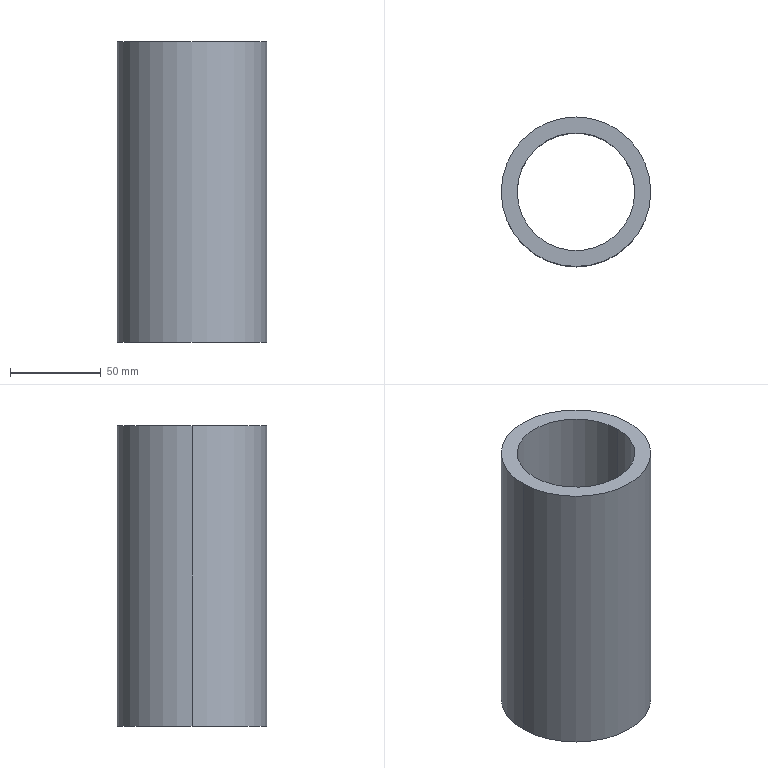Part | SolidWorks | features Extrusion 1 | 1 solid | 6 faces | box 82.5 x 82.5 x 166 mm | volume 338227 mm3 | cylinder 4 | plane 2 | commonest cylinder face diameters 64.9 x2 82.5 x2
STEP:
#1=CARTESIAN_POINT('',(-32.45,0.,166.));
#2=VERTEX_POINT('',#1);
#3=CARTESIAN_POINT('',(32.45,0.,166.));
#4=VERTEX_POINT('',#3);
#5=CARTESIAN_POINT('',(0.,0.,166.));
#6=DIRECTION('',(0.,0.,1.));
#7=DIRECTION('',(1.,0.,0.));
#8=AXIS2_PLACEMENT_3D('',#5,#6,#7);
#9=CIRCLE('',#8,32.45);
#10=EDGE_CURVE('',#2,#4,#9,.T.);
#11=ORIENTED_EDGE('',*,*,#10,.T.);
#12=CARTESIAN_POINT('',(32.45,0.,0.));
#13=VERTEX_POINT('',#12);
#14=CARTESIAN_POINT('',(32.45,0.,166.));
#15=DIRECTION('',(0.,0.,-1.));
#16=VECTOR('',#15,1000.);
#17=LINE('',#14,#16);
#18=EDGE_CURVE('',#4,#13,#17,.T.);
#19=ORIENTED_EDGE('',*,*,#18,.T.);
#20=CARTESIAN_POINT('',(-32.45,0.,0.));
#21=VERTEX_POINT('',#20);
#22=CARTESIAN_POINT('',(0.,0.,0.));
#23=DIRECTION('',(0.,0.,1.));
#24=DIRECTION('',(1.,0.,0.));
#25=AXIS2_PLACEMENT_3D('',#22,#23,#24);
#26=CIRCLE('',#25,32.45);
#27=EDGE_CURVE('',#21,#13,#26,.T.);
#28=ORIENTED_EDGE('',*,*,#27,.F.);
#29=CARTESIAN_POINT('',(-32.45,0.,166.));
#30=DIRECTION('',(0.,0.,-1.));
#31=VECTOR('',#30,1000.);
#32=LINE('',#29,#31);
#33=EDGE_CURVE('',#2,#21,#32,.T.);
#34=ORIENTED_EDGE('',*,*,#33,.F.);
#35=EDGE_LOOP('',(#11,#19,#28,#34));
#36=FACE_OUTER_BOUND('',#35,.T.);
#37=CARTESIAN_POINT('',(0.,0.,166.));
#38=DIRECTION('',(0.,0.,-1.));
#39=DIRECTION('',(-1.,0.,0.));
#40=AXIS2_PLACEMENT_3D('',#37,#38,#39);
#41=CYLINDRICAL_SURFACE('',#40,32.45);
#42=ADVANCED_FACE('',(#36),#41,.F.);
#43=CARTESIAN_POINT('',(41.25,0.,166.));
#44=VERTEX_POINT('',#43);
#45=CARTESIAN_POINT('',(-41.25,0.,166.));
#46=VERTEX_POINT('',#45);
#47=CARTESIAN_POINT('',(0.,0.,166.));
#48=DIRECTION('',(0.,0.,1.));
#49=DIRECTION('',(1.,0.,0.));
#50=AXIS2_PLACEMENT_3D('',#47,#48,#49);
#51=CIRCLE('',#50,41.25);
#52=EDGE_CURVE('',#44,#46,#51,.T.);
#53=ORIENTED_EDGE('',*,*,#52,.F.);
#54=CARTESIAN_POINT('',(41.25,0.,0.));
#55=VERTEX_POINT('',#54);
#56=CARTESIAN_POINT('',(41.25,0.,166.));
#57=DIRECTION('',(0.,0.,-1.));
#58=VECTOR('',#57,1000.);
#59=LINE('',#56,#58);
#60=EDGE_CURVE('',#44,#55,#59,.T.);
#61=ORIENTED_EDGE('',*,*,#60,.T.);
#62=CARTESIAN_POINT('',(-41.25,0.,0.));
#63=VERTEX_POINT('',#62);
#64=CARTESIAN_POINT('',(0.,0.,0.));
#65=DIRECTION('',(0.,0.,1.));
#66=DIRECTION('',(1.,0.,0.));
#67=AXIS2_PLACEMENT_3D('',#64,#65,#66);
#68=CIRCLE('',#67,41.25);
#69=EDGE_CURVE('',#55,#63,#68,.T.);
#70=ORIENTED_EDGE('',*,*,#69,.T.);
#71=CARTESIAN_POINT('',(-41.25,0.,166.));
#72=DIRECTION('',(0.,0.,-1.));
#73=VECTOR('',#72,1000.);
#74=LINE('',#71,#73);
#75=EDGE_CURVE('',#46,#63,#74,.T.);
#76=ORIENTED_EDGE('',*,*,#75,.F.);
#77=EDGE_LOOP('',(#53,#61,#70,#76));
#78=FACE_OUTER_BOUND('',#77,.T.);
#79=CARTESIAN_POINT('',(0.,0.,166.));
#80=DIRECTION('',(0.,0.,-1.));
#81=DIRECTION('',(-1.,0.,0.));
#82=AXIS2_PLACEMENT_3D('',#79,#80,#81);
#83=CYLINDRICAL_SURFACE('',#82,41.25);
#84=ADVANCED_FACE('',(#78),#83,.T.);
#85=CARTESIAN_POINT('',(0.,0.,166.));
#86=DIRECTION('',(0.,0.,1.));
#87=DIRECTION('',(1.,0.,0.));
#88=AXIS2_PLACEMENT_3D('',#85,#86,#87);
#89=CIRCLE('',#88,41.25);
#90=EDGE_CURVE('',#46,#44,#89,.T.);
#91=ORIENTED_EDGE('',*,*,#90,.T.);
#92=ORIENTED_EDGE('',*,*,#52,.T.);
#93=EDGE_LOOP('',(#91,#92));
#94=FACE_OUTER_BOUND('',#93,.T.);
#95=ORIENTED_EDGE('',*,*,#10,.F.);
#96=CARTESIAN_POINT('',(0.,0.,166.));
#97=DIRECTION('',(0.,0.,1.));
#98=DIRECTION('',(1.,0.,0.));
#99=AXIS2_PLACEMENT_3D('',#96,#97,#98);
#100=CIRCLE('',#99,32.45);
#101=EDGE_CURVE('',#4,#2,#100,.T.);
#102=ORIENTED_EDGE('',*,*,#101,.F.);
#103=EDGE_LOOP('',(#95,#102));
#104=FACE_BOUND('',#103,.T.);
#105=CARTESIAN_POINT('',(0.,0.,166.));
#106=DIRECTION('',(0.,0.,1.));
#107=DIRECTION('',(1.,0.,0.));
#108=AXIS2_PLACEMENT_3D('',#105,#106,#107);
#109=PLANE('',#108);
#110=ADVANCED_FACE('',(#94,#104),#109,.T.);
#111=CARTESIAN_POINT('',(0.,0.,0.));
#112=DIRECTION('',(0.,0.,1.));
#113=DIRECTION('',(1.,0.,0.));
#114=AXIS2_PLACEMENT_3D('',#111,#112,#113);
#115=CIRCLE('',#114,41.25);
#116=EDGE_CURVE('',#63,#55,#115,.T.);
#117=ORIENTED_EDGE('',*,*,#116,.F.);
#118=ORIENTED_EDGE('',*,*,#69,.F.);
#119=EDGE_LOOP('',(#117,#118));
#120=FACE_OUTER_BOUND('',#119,.T.);
#121=ORIENTED_EDGE('',*,*,#27,.T.);
#122=CARTESIAN_POINT('',(0.,0.,0.));
#123=DIRECTION('',(0.,0.,1.));
#124=DIRECTION('',(1.,0.,0.));
#125=AXIS2_PLACEMENT_3D('',#122,#123,#124);
#126=CIRCLE('',#125,32.45);
#127=EDGE_CURVE('',#13,#21,#126,.T.);
#128=ORIENTED_EDGE('',*,*,#127,.T.);
#129=EDGE_LOOP('',(#121,#128));
#130=FACE_BOUND('',#129,.T.);
#131=CARTESIAN_POINT('',(0.,0.,0.));
#132=DIRECTION('',(0.,0.,1.));
#133=DIRECTION('',(1.,0.,0.));
#134=AXIS2_PLACEMENT_3D('',#131,#132,#133);
#135=PLANE('',#134);
#136=ADVANCED_FACE('',(#120,#130),#135,.F.);
#137=ORIENTED_EDGE('',*,*,#60,.F.);
#138=ORIENTED_EDGE('',*,*,#90,.F.);
#139=ORIENTED_EDGE('',*,*,#75,.T.);
#140=ORIENTED_EDGE('',*,*,#116,.T.);
#141=EDGE_LOOP('',(#137,#138,#139,#140));
#142=FACE_OUTER_BOUND('',#141,.T.);
#143=CARTESIAN_POINT('',(0.,0.,166.));
#144=DIRECTION('',(0.,0.,-1.));
#145=DIRECTION('',(-1.,0.,0.));
#146=AXIS2_PLACEMENT_3D('',#143,#144,#145);
#147=CYLINDRICAL_SURFACE('',#146,41.25);
#148=ADVANCED_FACE('',(#142),#147,.T.);
#149=ORIENTED_EDGE('',*,*,#18,.F.);
#150=ORIENTED_EDGE('',*,*,#101,.T.);
#151=ORIENTED_EDGE('',*,*,#33,.T.);
#152=ORIENTED_EDGE('',*,*,#127,.F.);
#153=EDGE_LOOP('',(#149,#150,#151,#152));
#154=FACE_OUTER_BOUND('',#153,.T.);
#155=CARTESIAN_POINT('',(0.,0.,166.));
#156=DIRECTION('',(0.,0.,-1.));
#157=DIRECTION('',(-1.,0.,0.));
#158=AXIS2_PLACEMENT_3D('',#155,#156,#157);
#159=CYLINDRICAL_SURFACE('',#158,32.45);
#160=ADVANCED_FACE('',(#154),#159,.F.);
#161=CLOSED_SHELL('',(#42,#84,#110,#136,#148,#160));
#162=MANIFOLD_SOLID_BREP('',#161);
#163=CARTESIAN_POINT('',(0.,0.,0.));
#164=DIRECTION('',(0.,0.,1.));
#165=DIRECTION('',(1.,0.,0.));
#166=AXIS2_PLACEMENT_3D('',#163,#164,#165);
#167=(LENGTH_UNIT()NAMED_UNIT(*)SI_UNIT(.MILLI.,.METRE.));
#168=UNCERTAINTY_MEASURE_WITH_UNIT(LENGTH_MEASURE(0.00001),#167,'','');
#169=(NAMED_UNIT(*)PLANE_ANGLE_UNIT()SI_UNIT($,.RADIAN.));
#170=(NAMED_UNIT(*)SI_UNIT($,.STERADIAN.)SOLID_ANGLE_UNIT());
#171=(GEOMETRIC_REPRESENTATION_CONTEXT(3)GLOBAL_UNCERTAINTY_ASSIGNED_CONTEXT((#168))GLOBAL_UNIT_ASSIGNED_CONTEXT((#167,#169,#170))REPRESENTATION_CONTEXT('',''));
#172=ADVANCED_BREP_SHAPE_REPRESENTATION('',(#162,#166),#171);